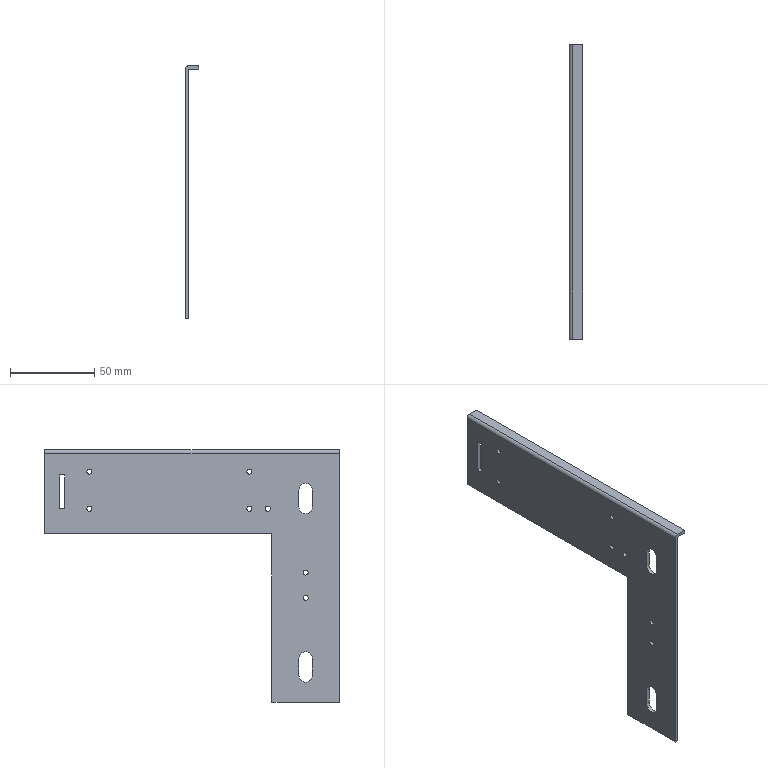Part | STEP file | 15 | 1 solid | 38 faces | box 8 x 175 x 150 mm | volume 26708 mm3 | cylinder 20 | plane 18 | commonest cylinder face diameters 3 x14 8 x4 0.02 x1 4.02 x1